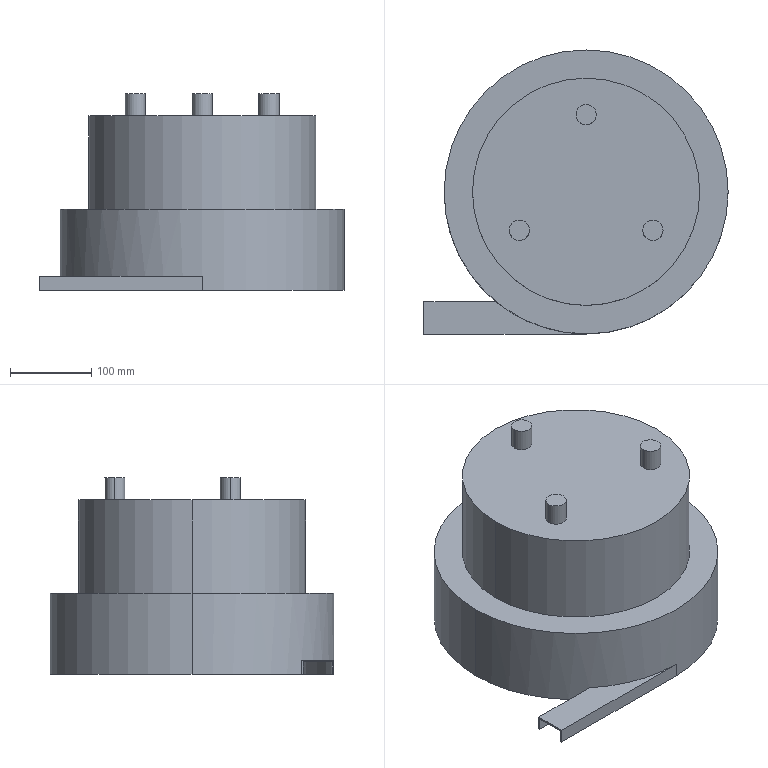Part | STEP file | Vibratory bowl | 1 solid | 29 faces | box 375 x 350 x 242.5 mm | volume 663388 mm3 | plane 15 | cylinder 14 | commonest cylinder face diameters 25 x6 276 x2 280 x2 346 x2 350 x2